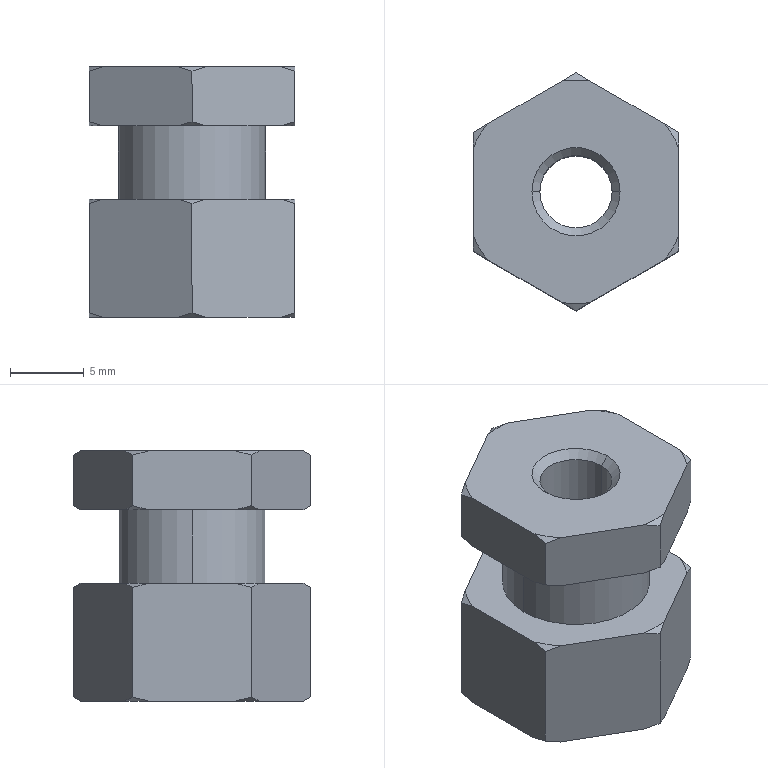Part | SolidWorks | features BaseBody 1 | 1 solid | 48 faces | box 14 x 16.166 x 17 mm | volume 2101 mm3 | cone 28 | plane 16 | cylinder 4 | commonest cylinder face diameters 4.917 x2 10 x2